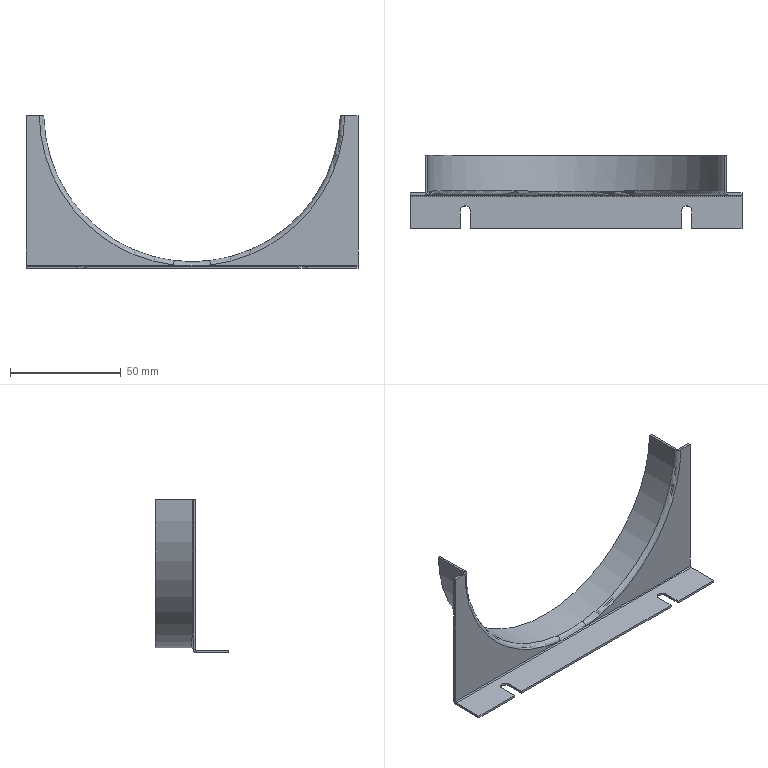Part | SolidWorks | features ICE 3, Fillet 2, EdgeFlange 1, FlatPattern 1, SMBaseFlange 1, SheetMetal 1 | 1 solid | 32 faces | box 150 x 33 x 69 mm | volume 8933 mm3 | plane 22 | cylinder 6 | torus 3 | spline 1 | commonest cylinder face diameters 4.5 x2 1 x1 3 x1 134 x1 136 x1
STEP:
#1=CARTESIAN_POINT('',(-52.25,-16.,-34.5));
#2=VERTEX_POINT('',#1);
#3=CARTESIAN_POINT('',(-75.,-16.,-34.5));
#4=VERTEX_POINT('',#3);
#5=CARTESIAN_POINT('',(0.,-16.,-34.5));
#6=DIRECTION('',(-1.,0.,0.));
#7=VECTOR('',#6,1000.);
#8=LINE('',#5,#7);
#9=EDGE_CURVE('',#2,#4,#8,.T.);
#10=ORIENTED_EDGE('',*,*,#9,.F.);
#11=CARTESIAN_POINT('',(-52.25,-16.,-33.5));
#12=VERTEX_POINT('',#11);
#13=CARTESIAN_POINT('',(-52.25,-16.,-34.5));
#14=DIRECTION('',(0.,0.,1.));
#15=VECTOR('',#14,1000.);
#16=LINE('',#13,#15);
#17=EDGE_CURVE('',#2,#12,#16,.T.);
#18=ORIENTED_EDGE('',*,*,#17,.T.);
#19=CARTESIAN_POINT('',(-75.,-16.,-33.5));
#20=VERTEX_POINT('',#19);
#21=CARTESIAN_POINT('',(-75.,-16.,-33.5));
#22=DIRECTION('',(-1.,0.,0.));
#23=VECTOR('',#22,1000.);
#24=LINE('',#21,#23);
#25=EDGE_CURVE('',#12,#20,#24,.T.);
#26=ORIENTED_EDGE('',*,*,#25,.T.);
#27=CARTESIAN_POINT('',(-75.,-16.,-34.5));
#28=DIRECTION('',(0.,0.,1.));
#29=VECTOR('',#28,1000.);
#30=LINE('',#27,#29);
#31=EDGE_CURVE('',#4,#20,#30,.T.);
#32=ORIENTED_EDGE('',*,*,#31,.F.);
#33=EDGE_LOOP('',(#10,#18,#26,#32));
#34=FACE_OUTER_BOUND('',#33,.T.);
#35=CARTESIAN_POINT('',(-75.,-16.,-34.5));
#36=DIRECTION('',(0.,1.,0.));
#37=DIRECTION('',(0.,0.,1.));
#38=AXIS2_PLACEMENT_3D('',#35,#36,#37);
#39=PLANE('',#38);
#40=ADVANCED_FACE('',(#34),#39,.F.);
#41=CARTESIAN_POINT('',(47.75,-16.,-33.5));
#42=VERTEX_POINT('',#41);
#43=CARTESIAN_POINT('',(-47.75,-16.,-33.5));
#44=VERTEX_POINT('',#43);
#45=CARTESIAN_POINT('',(-75.,-16.,-33.5));
#46=DIRECTION('',(-1.,0.,0.));
#47=VECTOR('',#46,1000.);
#48=LINE('',#45,#47);
#49=EDGE_CURVE('',#42,#44,#48,.T.);
#50=ORIENTED_EDGE('',*,*,#49,.T.);
#51=CARTESIAN_POINT('',(-47.75,-16.,-34.5));
#52=VERTEX_POINT('',#51);
#53=CARTESIAN_POINT('',(-47.75,-16.,-34.5));
#54=DIRECTION('',(0.,0.,1.));
#55=VECTOR('',#54,1000.);
#56=LINE('',#53,#55);
#57=EDGE_CURVE('',#52,#44,#56,.T.);
#58=ORIENTED_EDGE('',*,*,#57,.F.);
#59=CARTESIAN_POINT('',(47.75,-16.,-34.5));
#60=VERTEX_POINT('',#59);
#61=CARTESIAN_POINT('',(0.,-16.,-34.5));
#62=DIRECTION('',(-1.,0.,0.));
#63=VECTOR('',#62,1000.);
#64=LINE('',#61,#63);
#65=EDGE_CURVE('',#60,#52,#64,.T.);
#66=ORIENTED_EDGE('',*,*,#65,.F.);
#67=CARTESIAN_POINT('',(47.75,-16.,-34.5));
#68=DIRECTION('',(0.,0.,1.));
#69=VECTOR('',#68,1000.);
#70=LINE('',#67,#69);
#71=EDGE_CURVE('',#60,#42,#70,.T.);
#72=ORIENTED_EDGE('',*,*,#71,.T.);
#73=EDGE_LOOP('',(#50,#58,#66,#72));
#74=FACE_OUTER_BOUND('',#73,.T.);
#75=CARTESIAN_POINT('',(-75.,-16.,-34.5));
#76=DIRECTION('',(0.,1.,0.));
#77=DIRECTION('',(0.,0.,1.));
#78=AXIS2_PLACEMENT_3D('',#75,#76,#77);
#79=PLANE('',#78);
#80=ADVANCED_FACE('',(#74),#79,.F.);
#81=CARTESIAN_POINT('',(68.993,-1.,34.5));
#82=VERTEX_POINT('',#81);
#83=CARTESIAN_POINT('',(75.,-1.,34.5));
#84=VERTEX_POINT('',#83);
#85=CARTESIAN_POINT('',(-75.,-1.,34.5));
#86=DIRECTION('',(1.,0.,0.));
#87=VECTOR('',#86,1000.);
#88=LINE('',#85,#87);
#89=EDGE_CURVE('',#82,#84,#88,.T.);
#90=ORIENTED_EDGE('',*,*,#89,.F.);
#91=CARTESIAN_POINT('',(8.292,-1.,-33.));
#92=VERTEX_POINT('',#91);
#93=CARTESIAN_POINT('',(0.,-1.,35.5));
#94=DIRECTION('',(0.,1.,0.));
#95=DIRECTION('',(-1.,0.,0.));
#96=AXIS2_PLACEMENT_3D('',#93,#94,#95);
#97=CIRCLE('',#96,69.);
#98=EDGE_CURVE('',#82,#92,#97,.T.);
#99=ORIENTED_EDGE('',*,*,#98,.T.);
#100=CARTESIAN_POINT('',(75.,-1.,-33.));
#101=VERTEX_POINT('',#100);
#102=CARTESIAN_POINT('',(75.,-1.,-33.));
#103=DIRECTION('',(-1.,0.,0.));
#104=VECTOR('',#103,1000.);
#105=LINE('',#102,#104);
#106=EDGE_CURVE('',#101,#92,#105,.T.);
#107=ORIENTED_EDGE('',*,*,#106,.F.);
#108=CARTESIAN_POINT('',(75.,-1.,34.5));
#109=DIRECTION('',(0.,0.,-1.));
#110=VECTOR('',#109,1000.);
#111=LINE('',#108,#110);
#112=EDGE_CURVE('',#84,#101,#111,.T.);
#113=ORIENTED_EDGE('',*,*,#112,.F.);
#114=EDGE_LOOP('',(#90,#99,#107,#113));
#115=FACE_OUTER_BOUND('',#114,.T.);
#116=CARTESIAN_POINT('',(-75.,-1.,34.5));
#117=DIRECTION('',(0.,1.,0.));
#118=DIRECTION('',(-1.,0.,0.));
#119=AXIS2_PLACEMENT_3D('',#116,#117,#118);
#120=PLANE('',#119);
#121=ADVANCED_FACE('',(#115),#120,.F.);
#122=CARTESIAN_POINT('',(-75.,0.,34.5));
#123=VERTEX_POINT('',#122);
#124=CARTESIAN_POINT('',(-68.493,0.,34.5));
#125=VERTEX_POINT('',#124);
#126=CARTESIAN_POINT('',(-75.,0.,34.5));
#127=DIRECTION('',(1.,0.,0.));
#128=VECTOR('',#127,1000.);
#129=LINE('',#126,#128);
#130=EDGE_CURVE('',#123,#125,#129,.T.);
#131=ORIENTED_EDGE('',*,*,#130,.T.);
#132=CARTESIAN_POINT('',(0.,0.,-33.));
#133=VERTEX_POINT('',#132);
#134=CARTESIAN_POINT('',(0.,0.,35.5));
#135=DIRECTION('',(0.,-1.,0.));
#136=DIRECTION('',(-1.,0.,0.));
#137=AXIS2_PLACEMENT_3D('',#134,#135,#136);
#138=CIRCLE('',#137,68.5);
#139=EDGE_CURVE('',#125,#133,#138,.T.);
#140=ORIENTED_EDGE('',*,*,#139,.T.);
#141=CARTESIAN_POINT('',(-75.,0.,-33.));
#142=VERTEX_POINT('',#141);
#143=CARTESIAN_POINT('',(75.,0.,-33.));
#144=DIRECTION('',(-1.,0.,0.));
#145=VECTOR('',#144,1000.);
#146=LINE('',#143,#145);
#147=EDGE_CURVE('',#133,#142,#146,.T.);
#148=ORIENTED_EDGE('',*,*,#147,.T.);
#149=CARTESIAN_POINT('',(-75.,0.,34.5));
#150=DIRECTION('',(0.,0.,-1.));
#151=VECTOR('',#150,1000.);
#152=LINE('',#149,#151);
#153=EDGE_CURVE('',#123,#142,#152,.T.);
#154=ORIENTED_EDGE('',*,*,#153,.F.);
#155=EDGE_LOOP('',(#131,#140,#148,#154));
#156=FACE_OUTER_BOUND('',#155,.T.);
#157=CARTESIAN_POINT('',(-75.,0.,34.5));
#158=DIRECTION('',(0.,1.,0.));
#159=DIRECTION('',(-1.,0.,0.));
#160=AXIS2_PLACEMENT_3D('',#157,#158,#159);
#161=PLANE('',#160);
#162=ADVANCED_FACE('',(#156),#161,.T.);
#163=CARTESIAN_POINT('',(-8.292,-1.,-33.));
#164=VERTEX_POINT('',#163);
#165=CARTESIAN_POINT('',(-75.,-1.,-33.));
#166=VERTEX_POINT('',#165);
#167=CARTESIAN_POINT('',(75.,-1.,-33.));
#168=DIRECTION('',(-1.,0.,0.));
#169=VECTOR('',#168,1000.);
#170=LINE('',#167,#169);
#171=EDGE_CURVE('',#164,#166,#170,.T.);
#172=ORIENTED_EDGE('',*,*,#171,.F.);
#173=CARTESIAN_POINT('',(-68.993,-1.,34.5));
#174=VERTEX_POINT('',#173);
#175=CARTESIAN_POINT('',(0.,-1.,35.5));
#176=DIRECTION('',(0.,1.,0.));
#177=DIRECTION('',(-1.,0.,0.));
#178=AXIS2_PLACEMENT_3D('',#175,#176,#177);
#179=CIRCLE('',#178,69.);
#180=EDGE_CURVE('',#164,#174,#179,.T.);
#181=ORIENTED_EDGE('',*,*,#180,.T.);
#182=CARTESIAN_POINT('',(-75.,-1.,34.5));
#183=VERTEX_POINT('',#182);
#184=CARTESIAN_POINT('',(-75.,-1.,34.5));
#185=DIRECTION('',(1.,0.,0.));
#186=VECTOR('',#185,1000.);
#187=LINE('',#184,#186);
#188=EDGE_CURVE('',#183,#174,#187,.T.);
#189=ORIENTED_EDGE('',*,*,#188,.F.);
#190=CARTESIAN_POINT('',(-75.,-1.,34.5));
#191=DIRECTION('',(0.,0.,-1.));
#192=VECTOR('',#191,1000.);
#193=LINE('',#190,#192);
#194=EDGE_CURVE('',#183,#166,#193,.T.);
#195=ORIENTED_EDGE('',*,*,#194,.T.);
#196=EDGE_LOOP('',(#172,#181,#189,#195));
#197=FACE_OUTER_BOUND('',#196,.T.);
#198=CARTESIAN_POINT('',(-75.,-1.,34.5));
#199=DIRECTION('',(0.,1.,0.));
#200=DIRECTION('',(-1.,0.,0.));
#201=AXIS2_PLACEMENT_3D('',#198,#199,#200);
#202=PLANE('',#201);
#203=ADVANCED_FACE('',(#197),#202,.F.);
#204=ORIENTED_EDGE('',*,*,#112,.T.);
#205=CARTESIAN_POINT('',(75.,0.,-33.));
#206=VERTEX_POINT('',#205);
#207=CARTESIAN_POINT('',(75.,-1.,-33.));
#208=DIRECTION('',(0.,1.,0.));
#209=VECTOR('',#208,1000.);
#210=LINE('',#207,#209);
#211=EDGE_CURVE('',#101,#206,#210,.T.);
#212=ORIENTED_EDGE('',*,*,#211,.T.);
#213=CARTESIAN_POINT('',(75.,0.,34.5));
#214=VERTEX_POINT('',#213);
#215=CARTESIAN_POINT('',(75.,0.,34.5));
#216=DIRECTION('',(0.,0.,-1.));
#217=VECTOR('',#216,1000.);
#218=LINE('',#215,#217);
#219=EDGE_CURVE('',#214,#206,#218,.T.);
#220=ORIENTED_EDGE('',*,*,#219,.F.);
#221=CARTESIAN_POINT('',(75.,0.,34.5));
#222=DIRECTION('',(0.,-1.,0.));
#223=VECTOR('',#222,1000.);
#224=LINE('',#221,#223);
#225=EDGE_CURVE('',#214,#84,#224,.T.);
#226=ORIENTED_EDGE('',*,*,#225,.T.);
#227=EDGE_LOOP('',(#204,#212,#220,#226));
#228=FACE_OUTER_BOUND('',#227,.T.);
#229=CARTESIAN_POINT('',(75.,0.,34.5));
#230=DIRECTION('',(1.,0.,0.));
#231=DIRECTION('',(0.,0.,-1.));
#232=AXIS2_PLACEMENT_3D('',#229,#230,#231);
#233=PLANE('',#232);
#234=ADVANCED_FACE('',(#228),#233,.T.);
#235=CARTESIAN_POINT('',(75.,0.,-33.));
#236=DIRECTION('',(-1.,0.,0.));
#237=VECTOR('',#236,1000.);
#238=LINE('',#235,#237);
#239=EDGE_CURVE('',#206,#133,#238,.T.);
#240=ORIENTED_EDGE('',*,*,#239,.T.);
#241=CARTESIAN_POINT('',(68.493,0.,34.5));
#242=VERTEX_POINT('',#241);
#243=CARTESIAN_POINT('',(0.,0.,35.5));
#244=DIRECTION('',(0.,-1.,0.));
#245=DIRECTION('',(-1.,0.,0.));
#246=AXIS2_PLACEMENT_3D('',#243,#244,#245);
#247=CIRCLE('',#246,68.5);
#248=EDGE_CURVE('',#133,#242,#247,.T.);
#249=ORIENTED_EDGE('',*,*,#248,.T.);
#250=CARTESIAN_POINT('',(-75.,0.,34.5));
#251=DIRECTION('',(1.,0.,0.));
#252=VECTOR('',#251,1000.);
#253=LINE('',#250,#252);
#254=EDGE_CURVE('',#242,#214,#253,.T.);
#255=ORIENTED_EDGE('',*,*,#254,.T.);
#256=ORIENTED_EDGE('',*,*,#219,.T.);
#257=EDGE_LOOP('',(#240,#249,#255,#256));
#258=FACE_OUTER_BOUND('',#257,.T.);
#259=CARTESIAN_POINT('',(-75.,0.,34.5));
#260=DIRECTION('',(0.,1.,0.));
#261=DIRECTION('',(-1.,0.,0.));
#262=AXIS2_PLACEMENT_3D('',#259,#260,#261);
#263=PLANE('',#262);
#264=ADVANCED_FACE('',(#258),#263,.T.);
#265=ORIENTED_EDGE('',*,*,#188,.T.);
#266=CARTESIAN_POINT('',(-66.993,1.,34.5));
#267=VERTEX_POINT('',#266);
#268=CARTESIAN_POINT('',(-68.993,-1.,34.5));
#269=CARTESIAN_POINT('',(-68.861,-1.,34.5));
#270=CARTESIAN_POINT('',(-68.731,-0.9871,34.5));
#271=CARTESIAN_POINT('',(-68.475,-0.9363,34.5));
#272=CARTESIAN_POINT('',(-68.348,-0.8979,34.5));
#273=CARTESIAN_POINT('',(-68.106,-0.7976,34.5));
#274=CARTESIAN_POINT('',(-67.991,-0.7363,34.5));
#275=CARTESIAN_POINT('',(-67.774,-0.5913,34.5));
#276=CARTESIAN_POINT('',(-67.671,-0.5069,34.5));
#277=CARTESIAN_POINT('',(-67.394,-0.2304,34.5));
#278=CARTESIAN_POINT('',(-67.245,-0.0075,34.5));
#279=CARTESIAN_POINT('',(-67.046,0.4734,34.5));
#280=CARTESIAN_POINT('',(-66.993,0.7359,34.5));
#281=CARTESIAN_POINT('',(-66.993,1.,34.5));
#282=B_SPLINE_CURVE_WITH_KNOTS('',3,(#268,#269,#270,#271,#272,#273,#274,#275,#276,#277,#278,#279,#280,#281),.UNSPECIFIED.,.F.,.F.,(4,2,2,2,2,2,4),(0.,0.0003906,0.0007811,0.001172,0.001562,0.002343,0.003124),.UNSPECIFIED.);
#283=EDGE_CURVE('',#174,#267,#282,.T.);
#284=ORIENTED_EDGE('',*,*,#283,.T.);
#285=CARTESIAN_POINT('',(-66.993,17.,34.5));
#286=VERTEX_POINT('',#285);
#287=CARTESIAN_POINT('',(-66.993,17.,34.5));
#288=DIRECTION('',(0.,-1.,0.));
#289=VECTOR('',#288,1000.);
#290=LINE('',#287,#289);
#291=EDGE_CURVE('',#286,#267,#290,.T.);
#292=ORIENTED_EDGE('',*,*,#291,.F.);
#293=CARTESIAN_POINT('',(-67.993,17.,34.5));
#294=VERTEX_POINT('',#293);
#295=CARTESIAN_POINT('',(-67.993,17.,34.5));
#296=DIRECTION('',(1.,0.,0.));
#297=VECTOR('',#296,1000.);
#298=LINE('',#295,#297);
#299=EDGE_CURVE('',#294,#286,#298,.T.);
#300=ORIENTED_EDGE('',*,*,#299,.F.);
#301=CARTESIAN_POINT('',(-67.993,0.5,34.5));
#302=VERTEX_POINT('',#301);
#303=CARTESIAN_POINT('',(-67.993,17.,34.5));
#304=DIRECTION('',(0.,-1.,0.));
#305=VECTOR('',#304,1000.);
#306=LINE('',#303,#305);
#307=EDGE_CURVE('',#294,#302,#306,.T.);
#308=ORIENTED_EDGE('',*,*,#307,.T.);
#309=CARTESIAN_POINT('',(-67.993,0.5,34.5));
#310=CARTESIAN_POINT('',(-67.993,0.3679,34.5));
#311=CARTESIAN_POINT('',(-68.047,0.2388,34.5));
#312=CARTESIAN_POINT('',(-68.231,0.05433,34.5));
#313=CARTESIAN_POINT('',(-68.361,0.,34.5));
#314=CARTESIAN_POINT('',(-68.493,0.,34.5));
#315=B_SPLINE_CURVE_WITH_KNOTS('',3,(#309,#310,#311,#312,#313,#314),.UNSPECIFIED.,.F.,.F.,(4,2,4),(0.,0.0003906,0.0007811),.UNSPECIFIED.);
#316=EDGE_CURVE('',#302,#125,#315,.T.);
#317=ORIENTED_EDGE('',*,*,#316,.T.);
#318=ORIENTED_EDGE('',*,*,#130,.F.);
#319=CARTESIAN_POINT('',(-75.,-1.,34.5));
#320=DIRECTION('',(0.,1.,0.));
#321=VECTOR('',#320,1000.);
#322=LINE('',#319,#321);
#323=EDGE_CURVE('',#183,#123,#322,.T.);
#324=ORIENTED_EDGE('',*,*,#323,.F.);
#325=EDGE_LOOP('',(#265,#284,#292,#300,#308,#317,#318,#324));
#326=FACE_OUTER_BOUND('',#325,.T.);
#327=CARTESIAN_POINT('',(0.,0.,34.5));
#328=DIRECTION('',(0.,0.,-1.));
#329=DIRECTION('',(-1.,0.,0.));
#330=AXIS2_PLACEMENT_3D('',#327,#328,#329);
#331=PLANE('',#330);
#332=ADVANCED_FACE('',(#326),#331,.F.);
#333=CARTESIAN_POINT('',(-75.,-1.,-33.));
#334=DIRECTION('',(0.,1.,0.));
#335=VECTOR('',#334,1000.);
#336=LINE('',#333,#335);
#337=EDGE_CURVE('',#166,#142,#336,.T.);
#338=ORIENTED_EDGE('',*,*,#337,.F.);
#339=ORIENTED_EDGE('',*,*,#194,.F.);
#340=ORIENTED_EDGE('',*,*,#323,.T.);
#341=ORIENTED_EDGE('',*,*,#153,.T.);
#342=EDGE_LOOP('',(#338,#339,#340,#341));
#343=FACE_OUTER_BOUND('',#342,.T.);
#344=CARTESIAN_POINT('',(-75.,-1.,34.5));
#345=DIRECTION('',(-1.,0.,0.));
#346=DIRECTION('',(0.,0.,1.));
#347=AXIS2_PLACEMENT_3D('',#344,#345,#346);
#348=PLANE('',#347);
#349=ADVANCED_FACE('',(#343),#348,.T.);
#350=CARTESIAN_POINT('',(66.993,17.,34.5));
#351=VERTEX_POINT('',#350);
#352=CARTESIAN_POINT('',(66.993,1.,34.5));
#353=VERTEX_POINT('',#352);
#354=CARTESIAN_POINT('',(66.993,17.,34.5));
#355=DIRECTION('',(0.,-1.,0.));
#356=VECTOR('',#355,1000.);
#357=LINE('',#354,#356);
#358=EDGE_CURVE('',#351,#353,#357,.T.);
#359=ORIENTED_EDGE('',*,*,#358,.T.);
#360=CARTESIAN_POINT('',(66.993,1.,34.5));
#361=CARTESIAN_POINT('',(66.993,0.8679,34.5));
#362=CARTESIAN_POINT('',(67.005,0.7381,34.5));
#363=CARTESIAN_POINT('',(67.056,0.4826,34.5));
#364=CARTESIAN_POINT('',(67.095,0.3557,34.5));
#365=CARTESIAN_POINT('',(67.195,0.1136,34.5));
#366=CARTESIAN_POINT('',(67.256,-0.001272,34.5));
#367=CARTESIAN_POINT('',(67.401,-0.2186,34.5));
#368=CARTESIAN_POINT('',(67.486,-0.3215,34.5));
#369=CARTESIAN_POINT('',(67.762,-0.5982,34.5));
#370=CARTESIAN_POINT('',(67.985,-0.7473,34.5));
#371=CARTESIAN_POINT('',(68.466,-0.9469,34.5));
#372=CARTESIAN_POINT('',(68.729,-1.,34.5));
#373=CARTESIAN_POINT('',(68.993,-1.,34.5));
#374=B_SPLINE_CURVE_WITH_KNOTS('',3,(#360,#361,#362,#363,#364,#365,#366,#367,#368,#369,#370,#371,#372,#373),.UNSPECIFIED.,.F.,.F.,(4,2,2,2,2,2,4),(0.,0.0003906,0.0007811,0.001172,0.001562,0.002343,0.003124),.UNSPECIFIED.);
#375=EDGE_CURVE('',#353,#82,#374,.T.);
#376=ORIENTED_EDGE('',*,*,#375,.T.);
#377=ORIENTED_EDGE('',*,*,#89,.T.);
#378=ORIENTED_EDGE('',*,*,#225,.F.);
#379=ORIENTED_EDGE('',*,*,#254,.F.);
#380=CARTESIAN_POINT('',(67.993,0.5,34.5));
#381=VERTEX_POINT('',#380);
#382=CARTESIAN_POINT('',(68.493,0.,34.5));
#383=CARTESIAN_POINT('',(68.361,0.,34.5));
#384=CARTESIAN_POINT('',(68.231,0.05414,34.5));
#385=CARTESIAN_POINT('',(68.047,0.2385,34.5));
#386=CARTESIAN_POINT('',(67.993,0.3679,34.5));
#387=CARTESIAN_POINT('',(67.993,0.5,34.5));
#388=B_SPLINE_CURVE_WITH_KNOTS('',3,(#382,#383,#384,#385,#386,#387),.UNSPECIFIED.,.F.,.F.,(4,2,4),(0.,0.0003906,0.0007811),.UNSPECIFIED.);
#389=EDGE_CURVE('',#242,#381,#388,.T.);
#390=ORIENTED_EDGE('',*,*,#389,.T.);
#391=CARTESIAN_POINT('',(67.993,17.,34.5));
#392=VERTEX_POINT('',#391);
#393=CARTESIAN_POINT('',(67.993,17.,34.5));
#394=DIRECTION('',(0.,-1.,0.));
#395=VECTOR('',#394,1000.);
#396=LINE('',#393,#395);
#397=EDGE_CURVE('',#392,#381,#396,.T.);
#398=ORIENTED_EDGE('',*,*,#397,.F.);
#399=CARTESIAN_POINT('',(66.993,17.,34.5));
#400=DIRECTION('',(1.,0.,0.));
#401=VECTOR('',#400,1000.);
#402=LINE('',#399,#401);
#403=EDGE_CURVE('',#351,#392,#402,.T.);
#404=ORIENTED_EDGE('',*,*,#403,.F.);
#405=EDGE_LOOP('',(#359,#376,#377,#378,#379,#390,#398,#404));
#406=FACE_OUTER_BOUND('',#405,.T.);
#407=CARTESIAN_POINT('',(0.,0.,34.5));
#408=DIRECTION('',(0.,0.,-1.));
#409=DIRECTION('',(-1.,0.,0.));
#410=AXIS2_PLACEMENT_3D('',#407,#408,#409);
#411=PLANE('',#410);
#412=ADVANCED_FACE('',(#406),#411,.F.);
#413=ORIENTED_EDGE('',*,*,#291,.T.);
#414=CARTESIAN_POINT('',(-8.051,1.,-31.014));
#415=VERTEX_POINT('',#414);
#416=CARTESIAN_POINT('',(0.,1.,35.5));
#417=DIRECTION('',(0.,-1.,0.));
#418=DIRECTION('',(-1.,0.,0.));
#419=AXIS2_PLACEMENT_3D('',#416,#417,#418);
#420=CIRCLE('',#419,67.);
#421=EDGE_CURVE('',#267,#415,#420,.T.);
#422=ORIENTED_EDGE('',*,*,#421,.T.);
#423=CARTESIAN_POINT('',(8.051,1.,-31.014));
#424=VERTEX_POINT('',#423);
#425=CARTESIAN_POINT('',(-8.051,1.,-31.014));
#426=CARTESIAN_POINT('',(-6.713,1.,-31.176));
#427=CARTESIAN_POINT('',(-5.374,0.9844,-31.298));
#428=CARTESIAN_POINT('',(-2.693,0.9591,-31.459));
#429=CARTESIAN_POINT('',(-1.351,0.9495,-31.5));
#430=CARTESIAN_POINT('',(1.336,0.9495,-31.5));
#431=CARTESIAN_POINT('',(2.683,0.959,-31.46));
#432=CARTESIAN_POINT('',(5.372,0.9843,-31.298));
#433=CARTESIAN_POINT('',(6.713,1.,-31.176));
#434=CARTESIAN_POINT('',(8.051,1.,-31.014));
#435=B_SPLINE_CURVE_WITH_KNOTS('',3,(#425,#426,#427,#428,#429,#430,#431,#432,#433,#434),.UNSPECIFIED.,.F.,.F.,(4,2,2,2,4),(0.,0.004028,0.008056,0.01208,0.01611),.UNSPECIFIED.);
#436=EDGE_CURVE('',#415,#424,#435,.T.);
#437=ORIENTED_EDGE('',*,*,#436,.T.);
#438=CARTESIAN_POINT('',(0.,1.,35.5));
#439=DIRECTION('',(0.,-1.,0.));
#440=DIRECTION('',(-1.,0.,0.));
#441=AXIS2_PLACEMENT_3D('',#438,#439,#440);
#442=CIRCLE('',#441,67.);
#443=EDGE_CURVE('',#424,#353,#442,.T.);
#444=ORIENTED_EDGE('',*,*,#443,.T.);
#445=ORIENTED_EDGE('',*,*,#358,.F.);
#446=CARTESIAN_POINT('',(0.,17.,35.5));
#447=DIRECTION('',(0.,-1.,0.));
#448=DIRECTION('',(-1.,0.,0.));
#449=AXIS2_PLACEMENT_3D('',#446,#447,#448);
#450=CIRCLE('',#449,67.);
#451=EDGE_CURVE('',#286,#351,#450,.T.);
#452=ORIENTED_EDGE('',*,*,#451,.F.);
#453=EDGE_LOOP('',(#413,#422,#437,#444,#445,#452));
#454=FACE_OUTER_BOUND('',#453,.T.);
#455=CARTESIAN_POINT('',(0.,17.,35.5));
#456=DIRECTION('',(0.,-1.,0.));
#457=DIRECTION('',(1.,0.,0.));
#458=AXIS2_PLACEMENT_3D('',#455,#456,#457);
#459=CYLINDRICAL_SURFACE('',#458,67.);
#460=ADVANCED_FACE('',(#454),#459,.F.);
#461=ORIENTED_EDGE('',*,*,#397,.T.);
#462=CARTESIAN_POINT('',(0.,0.5,35.5));
#463=DIRECTION('',(0.,1.,0.));
#464=DIRECTION('',(-1.,0.,0.));
#465=AXIS2_PLACEMENT_3D('',#462,#463,#464);
#466=CIRCLE('',#465,68.);
#467=EDGE_CURVE('',#381,#302,#466,.T.);
#468=ORIENTED_EDGE('',*,*,#467,.T.);
#469=ORIENTED_EDGE('',*,*,#307,.F.);
#470=CARTESIAN_POINT('',(0.,17.,35.5));
#471=DIRECTION('',(0.,1.,0.));
#472=DIRECTION('',(-1.,0.,0.));
#473=AXIS2_PLACEMENT_3D('',#470,#471,#472);
#474=CIRCLE('',#473,68.);
#475=EDGE_CURVE('',#392,#294,#474,.T.);
#476=ORIENTED_EDGE('',*,*,#475,.F.);
#477=EDGE_LOOP('',(#461,#468,#469,#476));
#478=FACE_OUTER_BOUND('',#477,.T.);
#479=CARTESIAN_POINT('',(0.,17.,35.5));
#480=DIRECTION('',(0.,-1.,0.));
#481=DIRECTION('',(1.,0.,0.));
#482=AXIS2_PLACEMENT_3D('',#479,#480,#481);
#483=CYLINDRICAL_SURFACE('',#482,68.);
#484=ADVANCED_FACE('',(#478),#483,.T.);
#485=ORIENTED_EDGE('',*,*,#451,.T.);
#486=ORIENTED_EDGE('',*,*,#403,.T.);
#487=ORIENTED_EDGE('',*,*,#475,.T.);
#488=ORIENTED_EDGE('',*,*,#299,.T.);
#489=EDGE_LOOP('',(#485,#486,#487,#488));
#490=FACE_OUTER_BOUND('',#489,.T.);
#491=CARTESIAN_POINT('',(0.,17.,35.5));
#492=DIRECTION('',(0.,1.,0.));
#493=DIRECTION('',(-1.,0.,0.));
#494=AXIS2_PLACEMENT_3D('',#491,#492,#493);
#495=PLANE('',#494);
#496=ADVANCED_FACE('',(#490),#495,.T.);
#497=CARTESIAN_POINT('',(-75.,-1.5,-33.5));
#498=VERTEX_POINT('',#497);
#499=CARTESIAN_POINT('',(-75.,-1.5,-34.5));
#500=VERTEX_POINT('',#499);
#501=CARTESIAN_POINT('',(-75.,-1.5,-34.5));
#502=DIRECTION('',(0.,0.,-1.));
#503=VECTOR('',#502,1000.);
#504=LINE('',#501,#503);
#505=EDGE_CURVE('',#498,#500,#504,.T.);
#506=ORIENTED_EDGE('',*,*,#505,.F.);
#507=CARTESIAN_POINT('',(-75.,-1.5,-33.));
#508=DIRECTION('',(-1.,0.,0.));
#509=DIRECTION('',(0.,0.,-1.));
#510=AXIS2_PLACEMENT_3D('',#507,#508,#509);
#511=CIRCLE('',#510,0.5);
#512=EDGE_CURVE('',#166,#498,#511,.T.);
#513=ORIENTED_EDGE('',*,*,#512,.F.);
#514=ORIENTED_EDGE('',*,*,#337,.T.);
#515=CARTESIAN_POINT('',(-75.,-1.5,-33.));
#516=DIRECTION('',(-1.,0.,0.));
#517=DIRECTION('',(0.,0.,-1.));
#518=AXIS2_PLACEMENT_3D('',#515,#516,#517);
#519=CIRCLE('',#518,1.5);
#520=EDGE_CURVE('',#142,#500,#519,.T.);
#521=ORIENTED_EDGE('',*,*,#520,.T.);
#522=EDGE_LOOP('',(#506,#513,#514,#521));
#523=FACE_OUTER_BOUND('',#522,.T.);
#524=CARTESIAN_POINT('',(-75.,-1.5,-33.));
#525=DIRECTION('',(-1.,0.,0.));
#526=DIRECTION('',(0.,0.,1.));
#527=AXIS2_PLACEMENT_3D('',#524,#525,#526);
#528=PLANE('',#527);
#529=ADVANCED_FACE('',(#523),#528,.T.);
#530=CARTESIAN_POINT('',(75.,-1.5,-33.5));
#531=VERTEX_POINT('',#530);
#532=CARTESIAN_POINT('',(75.,-1.5,-33.));
#533=DIRECTION('',(1.,0.,0.));
#534=DIRECTION('',(0.,0.,-1.));
#535=AXIS2_PLACEMENT_3D('',#532,#533,#534);
#536=CIRCLE('',#535,0.5);
#537=EDGE_CURVE('',#531,#101,#536,.T.);
#538=ORIENTED_EDGE('',*,*,#537,.F.);
#539=CARTESIAN_POINT('',(75.,-1.5,-34.5));
#540=VERTEX_POINT('',#539);
#541=CARTESIAN_POINT('',(75.,-1.5,-33.5));
#542=DIRECTION('',(0.,0.,-1.));
#543=VECTOR('',#542,1000.);
#544=LINE('',#541,#543);
#545=EDGE_CURVE('',#531,#540,#544,.T.);
#546=ORIENTED_EDGE('',*,*,#545,.T.);
#547=CARTESIAN_POINT('',(75.,-1.5,-33.));
#548=DIRECTION('',(1.,0.,0.));
#549=DIRECTION('',(0.,0.,-1.));
#550=AXIS2_PLACEMENT_3D('',#547,#548,#549);
#551=CIRCLE('',#550,1.5);
#552=EDGE_CURVE('',#540,#206,#551,.T.);
#553=ORIENTED_EDGE('',*,*,#552,.T.);
#554=ORIENTED_EDGE('',*,*,#211,.F.);
#555=EDGE_LOOP('',(#538,#546,#553,#554));
#556=FACE_OUTER_BOUND('',#555,.T.);
#557=CARTESIAN_POINT('',(75.,-1.5,-33.));
#558=DIRECTION('',(-1.,0.,0.));
#559=DIRECTION('',(0.,0.,1.));
#560=AXIS2_PLACEMENT_3D('',#557,#558,#559);
#561=PLANE('',#560);
#562=ADVANCED_FACE('',(#556),#561,.F.);
#563=ORIENTED_EDGE('',*,*,#239,.F.);
#564=ORIENTED_EDGE('',*,*,#552,.F.);
#565=CARTESIAN_POINT('',(-75.,-1.5,-34.5));
#566=DIRECTION('',(-1.,0.,0.));
#567=VECTOR('',#566,1000.);
#568=LINE('',#565,#567);
#569=EDGE_CURVE('',#540,#500,#568,.T.);
#570=ORIENTED_EDGE('',*,*,#569,.T.);
#571=ORIENTED_EDGE('',*,*,#520,.F.);
#572=ORIENTED_EDGE('',*,*,#147,.F.);
#573=EDGE_LOOP('',(#563,#564,#570,#571,#572));
#574=FACE_OUTER_BOUND('',#573,.T.);
#575=CARTESIAN_POINT('',(75.,-1.5,-33.));
#576=DIRECTION('',(1.,0.,0.));
#577=DIRECTION('',(0.,0.,-1.));
#578=AXIS2_PLACEMENT_3D('',#575,#576,#577);
#579=CYLINDRICAL_SURFACE('',#578,1.5);
#580=ADVANCED_FACE('',(#574),#579,.T.);
#581=ORIENTED_EDGE('',*,*,#106,.T.);
#582=CARTESIAN_POINT('',(8.292,-1.,-33.));
#583=CARTESIAN_POINT('',(5.528,-1.,-33.067));
#584=CARTESIAN_POINT('',(2.764,-1.01,-33.1));
#585=CARTESIAN_POINT('',(-2.764,-1.01,-33.1));
#586=CARTESIAN_POINT('',(-5.528,-1.,-33.067));
#587=CARTESIAN_POINT('',(-8.292,-1.,-33.));
#588=B_SPLINE_CURVE_WITH_KNOTS('',3,(#582,#583,#584,#585,#586,#587),.UNSPECIFIED.,.F.,.F.,(4,2,4),(0.,0.008292,0.01658),.UNSPECIFIED.);
#589=EDGE_CURVE('',#92,#164,#588,.T.);
#590=ORIENTED_EDGE('',*,*,#589,.T.);
#591=ORIENTED_EDGE('',*,*,#171,.T.);
#592=ORIENTED_EDGE('',*,*,#512,.T.);
#593=CARTESIAN_POINT('',(-75.,-1.5,-33.5));
#594=DIRECTION('',(1.,0.,0.));
#595=VECTOR('',#594,1000.);
#596=LINE('',#593,#595);
#597=EDGE_CURVE('',#498,#531,#596,.T.);
#598=ORIENTED_EDGE('',*,*,#597,.T.);
#599=ORIENTED_EDGE('',*,*,#537,.T.);
#600=EDGE_LOOP('',(#581,#590,#591,#592,#598,#599));
#601=FACE_OUTER_BOUND('',#600,.T.);
#602=CARTESIAN_POINT('',(75.,-1.5,-33.));
#603=DIRECTION('',(1.,0.,0.));
#604=DIRECTION('',(0.,0.,-1.));
#605=AXIS2_PLACEMENT_3D('',#602,#603,#604);
#606=CYLINDRICAL_SURFACE('',#605,0.5);
#607=ADVANCED_FACE('',(#601),#606,.F.);
#608=ORIENTED_EDGE('',*,*,#505,.T.);
#609=CARTESIAN_POINT('',(-75.,0.,-34.5));
#610=DIRECTION('',(0.,1.,0.));
#611=VECTOR('',#610,1000.);
#612=LINE('',#609,#611);
#613=EDGE_CURVE('',#4,#500,#612,.T.);
#614=ORIENTED_EDGE('',*,*,#613,.F.);
#615=ORIENTED_EDGE('',*,*,#31,.T.);
#616=CARTESIAN_POINT('',(-75.,-1.,-33.5));
#617=DIRECTION('',(0.,1.,0.));
#618=VECTOR('',#617,1000.);
#619=LINE('',#616,#618);
#620=EDGE_CURVE('',#20,#498,#619,.T.);
#621=ORIENTED_EDGE('',*,*,#620,.T.);
#622=EDGE_LOOP('',(#608,#614,#615,#621));
#623=FACE_OUTER_BOUND('',#622,.T.);
#624=CARTESIAN_POINT('',(-75.,-1.,-34.5));
#625=DIRECTION('',(1.,0.,0.));
#626=DIRECTION('',(0.,0.,-1.));
#627=AXIS2_PLACEMENT_3D('',#624,#625,#626);
#628=PLANE('',#627);
#629=ADVANCED_FACE('',(#623),#628,.F.);
#630=ORIENTED_EDGE('',*,*,#545,.F.);
#631=CARTESIAN_POINT('',(75.,-16.,-33.5));
#632=VERTEX_POINT('',#631);
#633=CARTESIAN_POINT('',(75.,-16.,-33.5));
#634=DIRECTION('',(0.,-1.,0.));
#635=VECTOR('',#634,1000.);
#636=LINE('',#633,#635);
#637=EDGE_CURVE('',#531,#632,#636,.T.);
#638=ORIENTED_EDGE('',*,*,#637,.T.);
#639=CARTESIAN_POINT('',(75.,-16.,-34.5));
#640=VERTEX_POINT('',#639);
#641=CARTESIAN_POINT('',(75.,-16.,-34.5));
#642=DIRECTION('',(0.,0.,1.));
#643=VECTOR('',#642,1000.);
#644=LINE('',#641,#643);
#645=EDGE_CURVE('',#640,#632,#644,.T.);
#646=ORIENTED_EDGE('',*,*,#645,.F.);
#647=CARTESIAN_POINT('',(75.,0.,-34.5));
#648=DIRECTION('',(0.,-1.,0.));
#649=VECTOR('',#648,1000.);
#650=LINE('',#647,#649);
#651=EDGE_CURVE('',#540,#640,#650,.T.);
#652=ORIENTED_EDGE('',*,*,#651,.F.);
#653=EDGE_LOOP('',(#630,#638,#646,#652));
#654=FACE_OUTER_BOUND('',#653,.T.);
#655=CARTESIAN_POINT('',(75.,-16.,-34.5));
#656=DIRECTION('',(-1.,0.,0.));
#657=DIRECTION('',(0.,0.,1.));
#658=AXIS2_PLACEMENT_3D('',#655,#656,#657);
#659=PLANE('',#658);
#660=ADVANCED_FACE('',(#654),#659,.F.);
#661=CARTESIAN_POINT('',(-47.75,-8.,-34.5));
#662=VERTEX_POINT('',#661);
#663=CARTESIAN_POINT('',(-52.25,-8.,-34.5));
#664=VERTEX_POINT('',#663);
#665=CARTESIAN_POINT('',(-50.,-8.,-34.5));
#666=DIRECTION('',(0.,0.,1.));
#667=DIRECTION('',(1.,0.,0.));
#668=AXIS2_PLACEMENT_3D('',#665,#666,#667);
#669=CIRCLE('',#668,2.25);
#670=EDGE_CURVE('',#662,#664,#669,.T.);
#671=ORIENTED_EDGE('',*,*,#670,.T.);
#672=CARTESIAN_POINT('',(-52.25,-16.,-34.5));
#673=DIRECTION('',(0.,-1.,0.));
#674=VECTOR('',#673,1000.);
#675=LINE('',#672,#674);
#676=EDGE_CURVE('',#664,#2,#675,.T.);
#677=ORIENTED_EDGE('',*,*,#676,.T.);
#678=ORIENTED_EDGE('',*,*,#9,.T.);
#679=ORIENTED_EDGE('',*,*,#613,.T.);
#680=ORIENTED_EDGE('',*,*,#569,.F.);
#681=ORIENTED_EDGE('',*,*,#651,.T.);
#682=CARTESIAN_POINT('',(52.25,-16.,-34.5));
#683=VERTEX_POINT('',#682);
#684=CARTESIAN_POINT('',(0.,-16.,-34.5));
#685=DIRECTION('',(-1.,0.,0.));
#686=VECTOR('',#685,1000.);
#687=LINE('',#684,#686);
#688=EDGE_CURVE('',#640,#683,#687,.T.);
#689=ORIENTED_EDGE('',*,*,#688,.T.);
#690=CARTESIAN_POINT('',(52.25,-8.,-34.5));
#691=VERTEX_POINT('',#690);
#692=CARTESIAN_POINT('',(52.25,-16.,-34.5));
#693=DIRECTION('',(0.,1.,0.));
#694=VECTOR('',#693,1000.);
#695=LINE('',#692,#694);
#696=EDGE_CURVE('',#683,#691,#695,.T.);
#697=ORIENTED_EDGE('',*,*,#696,.T.);
#698=CARTESIAN_POINT('',(47.75,-8.,-34.5));
#699=VERTEX_POINT('',#698);
#700=CARTESIAN_POINT('',(50.,-8.,-34.5));
#701=DIRECTION('',(0.,0.,1.));
#702=DIRECTION('',(-1.,0.,0.));
#703=AXIS2_PLACEMENT_3D('',#700,#701,#702);
#704=CIRCLE('',#703,2.25);
#705=EDGE_CURVE('',#691,#699,#704,.T.);
#706=ORIENTED_EDGE('',*,*,#705,.T.);
#707=CARTESIAN_POINT('',(47.75,-16.,-34.5));
#708=DIRECTION('',(0.,-1.,0.));
#709=VECTOR('',#708,1000.);
#710=LINE('',#707,#709);
#711=EDGE_CURVE('',#699,#60,#710,.T.);
#712=ORIENTED_EDGE('',*,*,#711,.T.);
#713=ORIENTED_EDGE('',*,*,#65,.T.);
#714=CARTESIAN_POINT('',(-47.75,-16.,-34.5));
#715=DIRECTION('',(0.,1.,0.));
#716=VECTOR('',#715,1000.);
#717=LINE('',#714,#716);
#718=EDGE_CURVE('',#52,#662,#717,.T.);
#719=ORIENTED_EDGE('',*,*,#718,.T.);
#720=EDGE_LOOP('',(#671,#677,#678,#679,#680,#681,#689,#697,#706,#712,#713,#719));
#721=FACE_OUTER_BOUND('',#720,.T.);
#722=CARTESIAN_POINT('',(0.,0.,-34.5));
#723=DIRECTION('',(0.,0.,1.));
#724=DIRECTION('',(0.,-1.,0.));
#725=AXIS2_PLACEMENT_3D('',#722,#723,#724);
#726=PLANE('',#725);
#727=ADVANCED_FACE('',(#721),#726,.F.);
#728=CARTESIAN_POINT('',(-52.25,-8.,-33.5));
#729=VERTEX_POINT('',#728);
#730=CARTESIAN_POINT('',(-52.25,-16.,-33.5));
#731=DIRECTION('',(0.,-1.,0.));
#732=VECTOR('',#731,1000.);
#733=LINE('',#730,#732);
#734=EDGE_CURVE('',#729,#12,#733,.T.);
#735=ORIENTED_EDGE('',*,*,#734,.F.);
#736=CARTESIAN_POINT('',(-47.75,-8.,-33.5));
#737=VERTEX_POINT('',#736);
#738=CARTESIAN_POINT('',(-50.,-8.,-33.5));
#739=DIRECTION('',(0.,0.,1.));
#740=DIRECTION('',(1.,0.,0.));
#741=AXIS2_PLACEMENT_3D('',#738,#739,#740);
#742=CIRCLE('',#741,2.25);
#743=EDGE_CURVE('',#737,#729,#742,.T.);
#744=ORIENTED_EDGE('',*,*,#743,.F.);
#745=CARTESIAN_POINT('',(-47.75,-16.,-33.5));
#746=DIRECTION('',(0.,1.,0.));
#747=VECTOR('',#746,1000.);
#748=LINE('',#745,#747);
#749=EDGE_CURVE('',#44,#737,#748,.T.);
#750=ORIENTED_EDGE('',*,*,#749,.F.);
#751=ORIENTED_EDGE('',*,*,#49,.F.);
#752=CARTESIAN_POINT('',(47.75,-8.,-33.5));
#753=VERTEX_POINT('',#752);
#754=CARTESIAN_POINT('',(47.75,-16.,-33.5));
#755=DIRECTION('',(0.,-1.,0.));
#756=VECTOR('',#755,1000.);
#757=LINE('',#754,#756);
#758=EDGE_CURVE('',#753,#42,#757,.T.);
#759=ORIENTED_EDGE('',*,*,#758,.F.);
#760=CARTESIAN_POINT('',(52.25,-8.,-33.5));
#761=VERTEX_POINT('',#760);
#762=CARTESIAN_POINT('',(50.,-8.,-33.5));
#763=DIRECTION('',(0.,0.,1.));
#764=DIRECTION('',(-1.,0.,0.));
#765=AXIS2_PLACEMENT_3D('',#762,#763,#764);
#766=CIRCLE('',#765,2.25);
#767=EDGE_CURVE('',#761,#753,#766,.T.);
#768=ORIENTED_EDGE('',*,*,#767,.F.);
#769=CARTESIAN_POINT('',(52.25,-16.,-33.5));
#770=VERTEX_POINT('',#769);
#771=CARTESIAN_POINT('',(52.25,-16.,-33.5));
#772=DIRECTION('',(0.,1.,0.));
#773=VECTOR('',#772,1000.);
#774=LINE('',#771,#773);
#775=EDGE_CURVE('',#770,#761,#774,.T.);
#776=ORIENTED_EDGE('',*,*,#775,.F.);
#777=CARTESIAN_POINT('',(-75.,-16.,-33.5));
#778=DIRECTION('',(-1.,0.,0.));
#779=VECTOR('',#778,1000.);
#780=LINE('',#777,#779);
#781=EDGE_CURVE('',#632,#770,#780,.T.);
#782=ORIENTED_EDGE('',*,*,#781,.F.);
#783=ORIENTED_EDGE('',*,*,#637,.F.);
#784=ORIENTED_EDGE('',*,*,#597,.F.);
#785=ORIENTED_EDGE('',*,*,#620,.F.);
#786=ORIENTED_EDGE('',*,*,#25,.F.);
#787=EDGE_LOOP('',(#735,#744,#750,#751,#759,#768,#776,#782,#783,#784,#785,#786));
#788=FACE_OUTER_BOUND('',#787,.T.);
#789=CARTESIAN_POINT('',(0.,0.,-33.5));
#790=DIRECTION('',(0.,0.,1.));
#791=DIRECTION('',(0.,-1.,0.));
#792=AXIS2_PLACEMENT_3D('',#789,#790,#791);
#793=PLANE('',#792);
#794=ADVANCED_FACE('',(#788),#793,.T.);
#795=ORIENTED_EDGE('',*,*,#781,.T.);
#796=CARTESIAN_POINT('',(52.25,-16.,-34.5));
#797=DIRECTION('',(0.,0.,1.));
#798=VECTOR('',#797,1000.);
#799=LINE('',#796,#798);
#800=EDGE_CURVE('',#683,#770,#799,.T.);
#801=ORIENTED_EDGE('',*,*,#800,.F.);
#802=ORIENTED_EDGE('',*,*,#688,.F.);
#803=ORIENTED_EDGE('',*,*,#645,.T.);
#804=EDGE_LOOP('',(#795,#801,#802,#803));
#805=FACE_OUTER_BOUND('',#804,.T.);
#806=CARTESIAN_POINT('',(-75.,-16.,-34.5));
#807=DIRECTION('',(0.,1.,0.));
#808=DIRECTION('',(0.,0.,1.));
#809=AXIS2_PLACEMENT_3D('',#806,#807,#808);
#810=PLANE('',#809);
#811=ADVANCED_FACE('',(#805),#810,.F.);
#812=ORIENTED_EDGE('',*,*,#248,.F.);
#813=ORIENTED_EDGE('',*,*,#139,.F.);
#814=ORIENTED_EDGE('',*,*,#316,.F.);
#815=ORIENTED_EDGE('',*,*,#467,.F.);
#816=ORIENTED_EDGE('',*,*,#389,.F.);
#817=EDGE_LOOP('',(#812,#813,#814,#815,#816));
#818=FACE_OUTER_BOUND('',#817,.T.);
#819=CARTESIAN_POINT('',(0.,0.5,35.5));
#820=DIRECTION('',(0.,1.,0.));
#821=DIRECTION('',(-1.,0.,0.));
#822=AXIS2_PLACEMENT_3D('',#819,#820,#821);
#823=TOROIDAL_SURFACE('',#822,68.5,0.5);
#824=ADVANCED_FACE('',(#818),#823,.F.);
#825=ORIENTED_EDGE('',*,*,#283,.F.);
#826=ORIENTED_EDGE('',*,*,#180,.F.);
#827=CARTESIAN_POINT('',(-8.292,1.,-33.));
#828=DIRECTION('',(0.9928,0.,-0.1202));
#829=DIRECTION('',(-0.1202,0.,-0.9928));
#830=AXIS2_PLACEMENT_3D('',#827,#828,#829);
#831=CIRCLE('',#830,2.);
#832=EDGE_CURVE('',#415,#164,#831,.T.);
#833=ORIENTED_EDGE('',*,*,#832,.F.);
#834=ORIENTED_EDGE('',*,*,#421,.F.);
#835=EDGE_LOOP('',(#825,#826,#833,#834));
#836=FACE_OUTER_BOUND('',#835,.T.);
#837=CARTESIAN_POINT('',(0.,1.,35.5));
#838=DIRECTION('',(0.,1.,0.));
#839=DIRECTION('',(-1.,0.,0.));
#840=AXIS2_PLACEMENT_3D('',#837,#838,#839);
#841=TOROIDAL_SURFACE('',#840,69.,2.);
#842=ADVANCED_FACE('',(#836),#841,.T.);
#843=ORIENTED_EDGE('',*,*,#832,.T.);
#844=ORIENTED_EDGE('',*,*,#589,.F.);
#845=CARTESIAN_POINT('',(8.292,1.,-33.));
#846=DIRECTION('',(0.9928,0.,0.1202));
#847=DIRECTION('',(0.1202,0.,-0.9928));
#848=AXIS2_PLACEMENT_3D('',#845,#846,#847);
#849=CIRCLE('',#848,2.);
#850=EDGE_CURVE('',#424,#92,#849,.T.);
#851=ORIENTED_EDGE('',*,*,#850,.F.);
#852=ORIENTED_EDGE('',*,*,#436,.F.);
#853=EDGE_LOOP('',(#843,#844,#851,#852));
#854=FACE_OUTER_BOUND('',#853,.T.);
#855=CARTESIAN_POINT('',(8.051,1.,-31.014));
#856=CARTESIAN_POINT('',(8.051,-1.,-31.014));
#857=CARTESIAN_POINT('',(8.292,-1.,-33.));
#858=CARTESIAN_POINT('',(6.713,1.,-31.176));
#859=CARTESIAN_POINT('',(6.771,-0.8718,-31.169));
#860=CARTESIAN_POINT('',(6.914,-1.,-33.033));
#861=CARTESIAN_POINT('',(5.372,0.9843,-31.298));
#862=CARTESIAN_POINT('',(5.41,-0.7949,-31.295));
#863=CARTESIAN_POINT('',(5.533,-1.003,-33.058));
#864=CARTESIAN_POINT('',(2.683,0.959,-31.46));
#865=CARTESIAN_POINT('',(2.716,-0.7025,-31.458));
#866=CARTESIAN_POINT('',(2.763,-1.008,-33.092));
#867=CARTESIAN_POINT('',(1.336,0.9495,-31.5));
#868=CARTESIAN_POINT('',(1.343,-0.6834,-31.5));
#869=CARTESIAN_POINT('',(1.376,-1.01,-33.1));
#870=CARTESIAN_POINT('',(-1.351,0.9495,-31.5));
#871=CARTESIAN_POINT('',(-1.358,-0.6836,-31.5));
#872=CARTESIAN_POINT('',(-1.391,-1.01,-33.1));
#873=CARTESIAN_POINT('',(-2.693,0.9591,-31.459));
#874=CARTESIAN_POINT('',(-2.726,-0.7027,-31.458));
#875=CARTESIAN_POINT('',(-2.773,-1.008,-33.092));
#876=CARTESIAN_POINT('',(-5.374,0.9844,-31.298));
#877=CARTESIAN_POINT('',(-5.412,-0.7951,-31.295));
#878=CARTESIAN_POINT('',(-5.535,-1.003,-33.058));
#879=CARTESIAN_POINT('',(-6.713,1.,-31.176));
#880=CARTESIAN_POINT('',(-6.771,-0.8718,-31.169));
#881=CARTESIAN_POINT('',(-6.914,-1.,-33.033));
#882=CARTESIAN_POINT('',(-8.051,1.,-31.014));
#883=CARTESIAN_POINT('',(-8.051,-1.,-31.014));
#884=CARTESIAN_POINT('',(-8.292,-1.,-33.));
#885=(BOUNDED_SURFACE()B_SPLINE_SURFACE(3,2,((#855,#856,#857),(#858,#859,#860),(#861,#862,#863),(#864,#865,#866),(#867,#868,#869),(#870,#871,#872),(#873,#874,#875),(#876,#877,#878),(#879,#880,#881),(#882,#883,#884)),.UNSPECIFIED.,.F.,.F.,.T.)B_SPLINE_SURFACE_WITH_KNOTS((4,2,2,2,4),(3,3),(0.,0.004161,0.008321,0.01248,0.01664),(0.,1.),.UNSPECIFIED.)GEOMETRIC_REPRESENTATION_ITEM()RATIONAL_B_SPLINE_SURFACE(((1.,0.7071,1.),(1.,0.7305,1.),(1.,0.7472,1.),(1.,0.7693,1.),(1.,0.7746,1.),(1.,0.7746,1.),(1.,0.7692,1.),(1.,0.7472,1.),(1.,0.7305,1.),(1.,0.7071,1.)))REPRESENTATION_ITEM('')SURFACE());
#886=ADVANCED_FACE('',(#854),#885,.T.);
#887=ORIENTED_EDGE('',*,*,#375,.F.);
#888=ORIENTED_EDGE('',*,*,#443,.F.);
#889=ORIENTED_EDGE('',*,*,#850,.T.);
#890=ORIENTED_EDGE('',*,*,#98,.F.);
#891=EDGE_LOOP('',(#887,#888,#889,#890));
#892=FACE_OUTER_BOUND('',#891,.T.);
#893=CARTESIAN_POINT('',(0.,1.,35.5));
#894=DIRECTION('',(0.,1.,0.));
#895=DIRECTION('',(-1.,0.,0.));
#896=AXIS2_PLACEMENT_3D('',#893,#894,#895);
#897=TOROIDAL_SURFACE('',#896,69.,2.);
#898=ADVANCED_FACE('',(#892),#897,.T.);
#899=ORIENTED_EDGE('',*,*,#758,.T.);
#900=ORIENTED_EDGE('',*,*,#71,.F.);
#901=ORIENTED_EDGE('',*,*,#711,.F.);
#902=CARTESIAN_POINT('',(47.75,-8.,-34.5));
#903=DIRECTION('',(0.,0.,1.));
#904=VECTOR('',#903,1000.);
#905=LINE('',#902,#904);
#906=EDGE_CURVE('',#699,#753,#905,.T.);
#907=ORIENTED_EDGE('',*,*,#906,.T.);
#908=EDGE_LOOP('',(#899,#900,#901,#907));
#909=FACE_OUTER_BOUND('',#908,.T.);
#910=CARTESIAN_POINT('',(47.75,-16.,-34.5));
#911=DIRECTION('',(-1.,0.,0.));
#912=DIRECTION('',(0.,-1.,0.));
#913=AXIS2_PLACEMENT_3D('',#910,#911,#912);
#914=PLANE('',#913);
#915=ADVANCED_FACE('',(#909),#914,.F.);
#916=ORIENTED_EDGE('',*,*,#767,.T.);
#917=ORIENTED_EDGE('',*,*,#906,.F.);
#918=ORIENTED_EDGE('',*,*,#705,.F.);
#919=CARTESIAN_POINT('',(52.25,-8.,-34.5));
#920=DIRECTION('',(0.,0.,1.));
#921=VECTOR('',#920,1000.);
#922=LINE('',#919,#921);
#923=EDGE_CURVE('',#691,#761,#922,.T.);
#924=ORIENTED_EDGE('',*,*,#923,.T.);
#925=EDGE_LOOP('',(#916,#917,#918,#924));
#926=FACE_OUTER_BOUND('',#925,.T.);
#927=CARTESIAN_POINT('',(50.,-8.,-34.5));
#928=DIRECTION('',(0.,0.,1.));
#929=DIRECTION('',(1.,0.,0.));
#930=AXIS2_PLACEMENT_3D('',#927,#928,#929);
#931=CYLINDRICAL_SURFACE('',#930,2.25);
#932=ADVANCED_FACE('',(#926),#931,.F.);
#933=ORIENTED_EDGE('',*,*,#775,.T.);
#934=ORIENTED_EDGE('',*,*,#923,.F.);
#935=ORIENTED_EDGE('',*,*,#696,.F.);
#936=ORIENTED_EDGE('',*,*,#800,.T.);
#937=EDGE_LOOP('',(#933,#934,#935,#936));
#938=FACE_OUTER_BOUND('',#937,.T.);
#939=CARTESIAN_POINT('',(52.25,-16.,-34.5));
#940=DIRECTION('',(1.,0.,0.));
#941=DIRECTION('',(0.,1.,0.));
#942=AXIS2_PLACEMENT_3D('',#939,#940,#941);
#943=PLANE('',#942);
#944=ADVANCED_FACE('',(#938),#943,.F.);
#945=ORIENTED_EDGE('',*,*,#734,.T.);
#946=ORIENTED_EDGE('',*,*,#17,.F.);
#947=ORIENTED_EDGE('',*,*,#676,.F.);
#948=CARTESIAN_POINT('',(-52.25,-8.,-34.5));
#949=DIRECTION('',(0.,0.,1.));
#950=VECTOR('',#949,1000.);
#951=LINE('',#948,#950);
#952=EDGE_CURVE('',#664,#729,#951,.T.);
#953=ORIENTED_EDGE('',*,*,#952,.T.);
#954=EDGE_LOOP('',(#945,#946,#947,#953));
#955=FACE_OUTER_BOUND('',#954,.T.);
#956=CARTESIAN_POINT('',(-52.25,-16.,-34.5));
#957=DIRECTION('',(-1.,0.,0.));
#958=DIRECTION('',(0.,-1.,0.));
#959=AXIS2_PLACEMENT_3D('',#956,#957,#958);
#960=PLANE('',#959);
#961=ADVANCED_FACE('',(#955),#960,.F.);
#962=ORIENTED_EDGE('',*,*,#743,.T.);
#963=ORIENTED_EDGE('',*,*,#952,.F.);
#964=ORIENTED_EDGE('',*,*,#670,.F.);
#965=CARTESIAN_POINT('',(-47.75,-8.,-34.5));
#966=DIRECTION('',(0.,0.,1.));
#967=VECTOR('',#966,1000.);
#968=LINE('',#965,#967);
#969=EDGE_CURVE('',#662,#737,#968,.T.);
#970=ORIENTED_EDGE('',*,*,#969,.T.);
#971=EDGE_LOOP('',(#962,#963,#964,#970));
#972=FACE_OUTER_BOUND('',#971,.T.);
#973=CARTESIAN_POINT('',(-50.,-8.,-34.5));
#974=DIRECTION('',(0.,0.,1.));
#975=DIRECTION('',(1.,0.,0.));
#976=AXIS2_PLACEMENT_3D('',#973,#974,#975);
#977=CYLINDRICAL_SURFACE('',#976,2.25);
#978=ADVANCED_FACE('',(#972),#977,.F.);
#979=ORIENTED_EDGE('',*,*,#749,.T.);
#980=ORIENTED_EDGE('',*,*,#969,.F.);
#981=ORIENTED_EDGE('',*,*,#718,.F.);
#982=ORIENTED_EDGE('',*,*,#57,.T.);
#983=EDGE_LOOP('',(#979,#980,#981,#982));
#984=FACE_OUTER_BOUND('',#983,.T.);
#985=CARTESIAN_POINT('',(-47.75,-16.,-34.5));
#986=DIRECTION('',(1.,0.,0.));
#987=DIRECTION('',(0.,1.,0.));
#988=AXIS2_PLACEMENT_3D('',#985,#986,#987);
#989=PLANE('',#988);
#990=ADVANCED_FACE('',(#984),#989,.F.);
#991=CLOSED_SHELL('',(#40,#80,#121,#162,#203,#234,#264,#332,#349,#412,#460,#484,#496,#529,#562,#580,#607,#629,#660,#727,#794,#811,#824,#842,#886,#898,#915,#932,#944,#961,#978,#990));
#992=MANIFOLD_SOLID_BREP('',#991);
#993=CARTESIAN_POINT('',(0.,0.,0.));
#994=DIRECTION('',(0.,0.,1.));
#995=DIRECTION('',(1.,0.,0.));
#996=AXIS2_PLACEMENT_3D('',#993,#994,#995);
#997=(LENGTH_UNIT()NAMED_UNIT(*)SI_UNIT(.MILLI.,.METRE.));
#998=UNCERTAINTY_MEASURE_WITH_UNIT(LENGTH_MEASURE(0.00001),#997,'','');
#999=(NAMED_UNIT(*)PLANE_ANGLE_UNIT()SI_UNIT($,.RADIAN.));
#1000=(NAMED_UNIT(*)SI_UNIT($,.STERADIAN.)SOLID_ANGLE_UNIT());
#1001=(GEOMETRIC_REPRESENTATION_CONTEXT(3)GLOBAL_UNCERTAINTY_ASSIGNED_CONTEXT((#998))GLOBAL_UNIT_ASSIGNED_CONTEXT((#997,#999,#1000))REPRESENTATION_CONTEXT('',''));
#1002=ADVANCED_BREP_SHAPE_REPRESENTATION('',(#992,#996),#1001);